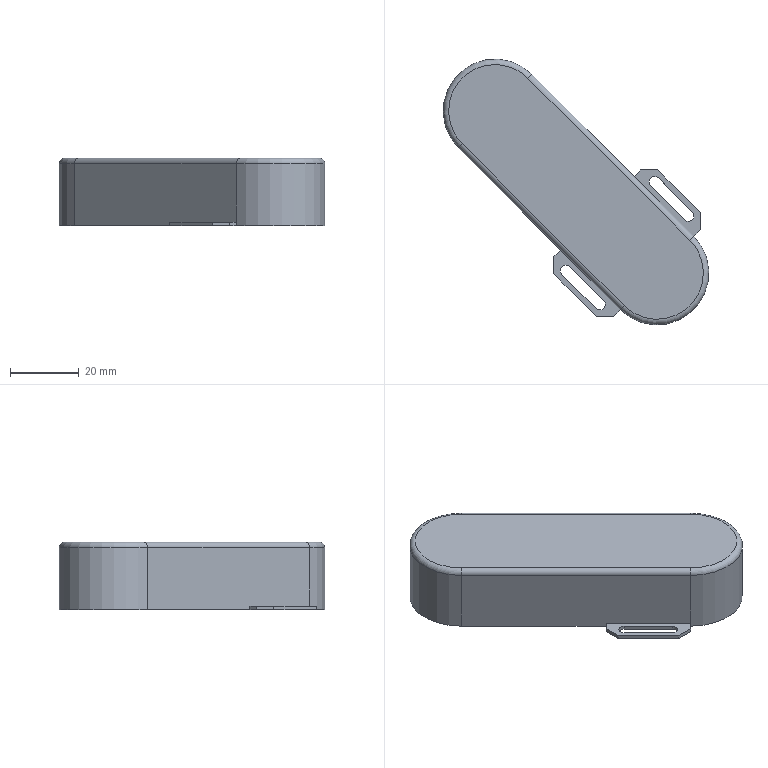Part | SolidWorks | features SplitBody 1 | 1 solid | 42 faces | box 77.123 x 77.123 x 19.6 mm | volume 7300 mm3 | plane 26 | cylinder 12 | torus 4 | commonest cylinder face diameters 3.15 x4 1.031 x2 3.131 x2 28 x2 30.1 x2
STEP:
#1=CARTESIAN_POINT('',(-32.023,223.663,-251.716));
#2=VERTEX_POINT('',#1);
#3=CARTESIAN_POINT('',(-32.023,223.663,-250.666));
#4=VERTEX_POINT('',#3);
#5=CARTESIAN_POINT('',(-32.023,223.663,-251.716));
#6=DIRECTION('',(0.,0.,1.));
#7=VECTOR('',#6,1000.);
#8=LINE('',#5,#7);
#9=EDGE_CURVE('',#2,#4,#8,.T.);
#10=ORIENTED_EDGE('',*,*,#9,.F.);
#11=CARTESIAN_POINT('',(-61.721,253.362,-251.716));
#12=VERTEX_POINT('',#11);
#13=CARTESIAN_POINT('',(-61.721,253.362,-251.716));
#14=DIRECTION('',(0.7071,-0.7071,0.));
#15=VECTOR('',#14,1000.);
#16=LINE('',#13,#15);
#17=EDGE_CURVE('',#12,#2,#16,.T.);
#18=ORIENTED_EDGE('',*,*,#17,.F.);
#19=CARTESIAN_POINT('',(-61.721,253.362,-233.681));
#20=VERTEX_POINT('',#19);
#21=CARTESIAN_POINT('',(-61.721,253.362,-233.166));
#22=DIRECTION('',(0.,0.,-1.));
#23=VECTOR('',#22,1000.);
#24=LINE('',#21,#23);
#25=EDGE_CURVE('',#20,#12,#24,.T.);
#26=ORIENTED_EDGE('',*,*,#25,.F.);
#27=CARTESIAN_POINT('',(-14.699,206.339,-233.681));
#28=VERTEX_POINT('',#27);
#29=CARTESIAN_POINT('',(-61.721,253.362,-233.681));
#30=DIRECTION('',(0.7071,-0.7071,0.));
#31=VECTOR('',#30,1000.);
#32=LINE('',#29,#31);
#33=EDGE_CURVE('',#20,#28,#32,.T.);
#34=ORIENTED_EDGE('',*,*,#33,.T.);
#35=CARTESIAN_POINT('',(-14.699,206.339,-250.666));
#36=VERTEX_POINT('',#35);
#37=CARTESIAN_POINT('',(-14.699,206.339,-233.166));
#38=DIRECTION('',(0.,0.,-1.));
#39=VECTOR('',#38,1000.);
#40=LINE('',#37,#39);
#41=EDGE_CURVE('',#28,#36,#40,.T.);
#42=ORIENTED_EDGE('',*,*,#41,.T.);
#43=CARTESIAN_POINT('',(-32.023,223.663,-250.666));
#44=DIRECTION('',(0.7071,-0.7071,0.));
#45=VECTOR('',#44,1000.);
#46=LINE('',#43,#45);
#47=EDGE_CURVE('',#4,#36,#46,.T.);
#48=ORIENTED_EDGE('',*,*,#47,.F.);
#49=EDGE_LOOP('',(#10,#18,#26,#34,#42,#48));
#50=FACE_OUTER_BOUND('',#49,.T.);
#51=CARTESIAN_POINT('',(-61.721,253.362,-233.166));
#52=DIRECTION('',(-0.7071,-0.7071,0.));
#53=DIRECTION('',(0.,0.,1.));
#54=AXIS2_PLACEMENT_3D('',#51,#52,#53);
#55=PLANE('',#54);
#56=ADVANCED_FACE('',(#50),#55,.F.);
#57=CARTESIAN_POINT('',(-35.983,185.055,-250.666));
#58=VERTEX_POINT('',#57);
#59=CARTESIAN_POINT('',(-53.307,202.379,-250.666));
#60=VERTEX_POINT('',#59);
#61=CARTESIAN_POINT('',(-53.307,202.379,-250.666));
#62=DIRECTION('',(-0.7071,0.7071,0.));
#63=VECTOR('',#62,1000.);
#64=LINE('',#61,#63);
#65=EDGE_CURVE('',#58,#60,#64,.T.);
#66=ORIENTED_EDGE('',*,*,#65,.F.);
#67=CARTESIAN_POINT('',(-35.983,185.055,-233.681));
#68=VERTEX_POINT('',#67);
#69=CARTESIAN_POINT('',(-35.983,185.055,-233.166));
#70=DIRECTION('',(0.,0.,-1.));
#71=VECTOR('',#70,1000.);
#72=LINE('',#69,#71);
#73=EDGE_CURVE('',#68,#58,#72,.T.);
#74=ORIENTED_EDGE('',*,*,#73,.F.);
#75=CARTESIAN_POINT('',(-83.005,232.078,-233.681));
#76=VERTEX_POINT('',#75);
#77=CARTESIAN_POINT('',(-35.983,185.055,-233.681));
#78=DIRECTION('',(-0.7071,0.7071,0.));
#79=VECTOR('',#78,1000.);
#80=LINE('',#77,#79);
#81=EDGE_CURVE('',#68,#76,#80,.T.);
#82=ORIENTED_EDGE('',*,*,#81,.T.);
#83=CARTESIAN_POINT('',(-83.005,232.078,-251.716));
#84=VERTEX_POINT('',#83);
#85=CARTESIAN_POINT('',(-83.005,232.078,-233.166));
#86=DIRECTION('',(0.,0.,-1.));
#87=VECTOR('',#86,1000.);
#88=LINE('',#85,#87);
#89=EDGE_CURVE('',#76,#84,#88,.T.);
#90=ORIENTED_EDGE('',*,*,#89,.T.);
#91=CARTESIAN_POINT('',(-53.307,202.379,-251.716));
#92=VERTEX_POINT('',#91);
#93=CARTESIAN_POINT('',(-35.983,185.055,-251.716));
#94=DIRECTION('',(-0.7071,0.7071,0.));
#95=VECTOR('',#94,1000.);
#96=LINE('',#93,#95);
#97=EDGE_CURVE('',#92,#84,#96,.T.);
#98=ORIENTED_EDGE('',*,*,#97,.F.);
#99=CARTESIAN_POINT('',(-53.307,202.379,-251.716));
#100=DIRECTION('',(0.,0.,-1.));
#101=VECTOR('',#100,1000.);
#102=LINE('',#99,#101);
#103=EDGE_CURVE('',#60,#92,#102,.T.);
#104=ORIENTED_EDGE('',*,*,#103,.F.);
#105=EDGE_LOOP('',(#66,#74,#82,#90,#98,#104));
#106=FACE_OUTER_BOUND('',#105,.T.);
#107=CARTESIAN_POINT('',(-35.983,185.055,-233.166));
#108=DIRECTION('',(0.7071,0.7071,0.));
#109=DIRECTION('',(0.,0.,-1.));
#110=AXIS2_PLACEMENT_3D('',#107,#108,#109);
#111=PLANE('',#110);
#112=ADVANCED_FACE('',(#106),#111,.F.);
#113=CARTESIAN_POINT('',(-82.263,232.82,-251.716));
#114=VERTEX_POINT('',#113);
#115=CARTESIAN_POINT('',(-82.263,232.82,-251.716));
#116=DIRECTION('',(0.7071,0.7071,0.));
#117=VECTOR('',#116,1000.);
#118=LINE('',#115,#117);
#119=EDGE_CURVE('',#84,#114,#118,.T.);
#120=ORIENTED_EDGE('',*,*,#119,.F.);
#121=CARTESIAN_POINT('',(-72.363,242.72,-251.716));
#122=DIRECTION('',(0.,0.,-1.));
#123=DIRECTION('',(-0.7071,-0.7071,0.));
#124=AXIS2_PLACEMENT_3D('',#121,#122,#123);
#125=CIRCLE('',#124,15.05);
#126=EDGE_CURVE('',#84,#12,#125,.T.);
#127=ORIENTED_EDGE('',*,*,#126,.T.);
#128=CARTESIAN_POINT('',(-62.464,252.619,-251.716));
#129=VERTEX_POINT('',#128);
#130=CARTESIAN_POINT('',(-62.464,252.619,-251.716));
#131=DIRECTION('',(-0.7071,-0.7071,0.));
#132=VECTOR('',#131,1000.);
#133=LINE('',#130,#132);
#134=EDGE_CURVE('',#12,#129,#133,.T.);
#135=ORIENTED_EDGE('',*,*,#134,.T.);
#136=CARTESIAN_POINT('',(-72.363,242.72,-251.716));
#137=DIRECTION('',(0.,0.,-1.));
#138=DIRECTION('',(-0.7071,-0.7071,0.));
#139=AXIS2_PLACEMENT_3D('',#136,#137,#138);
#140=CIRCLE('',#139,14.);
#141=EDGE_CURVE('',#114,#129,#140,.T.);
#142=ORIENTED_EDGE('',*,*,#141,.F.);
#143=EDGE_LOOP('',(#120,#127,#135,#142));
#144=FACE_OUTER_BOUND('',#143,.T.);
#145=CARTESIAN_POINT('',(-72.363,242.72,-251.716));
#146=DIRECTION('',(0.,0.,1.));
#147=DIRECTION('',(0.7071,0.7071,0.));
#148=AXIS2_PLACEMENT_3D('',#145,#146,#147);
#149=PLANE('',#148);
#150=ADVANCED_FACE('',(#144),#149,.F.);
#151=CARTESIAN_POINT('',(-27.197,221.064,-251.716));
#152=VERTEX_POINT('',#151);
#153=CARTESIAN_POINT('',(-24.97,223.292,-251.716));
#154=VERTEX_POINT('',#153);
#155=CARTESIAN_POINT('',(-26.083,222.178,-251.716));
#156=DIRECTION('',(0.,0.,-1.));
#157=DIRECTION('',(-0.7071,-0.7071,0.));
#158=AXIS2_PLACEMENT_3D('',#155,#156,#157);
#159=CIRCLE('',#158,1.575);
#160=EDGE_CURVE('',#152,#154,#159,.T.);
#161=ORIENTED_EDGE('',*,*,#160,.F.);
#162=CARTESIAN_POINT('',(-17.297,211.165,-251.716));
#163=VERTEX_POINT('',#162);
#164=CARTESIAN_POINT('',(-60.608,254.475,-251.716));
#165=DIRECTION('',(-0.7071,0.7071,0.));
#166=VECTOR('',#165,1000.);
#167=LINE('',#164,#166);
#168=EDGE_CURVE('',#163,#152,#167,.T.);
#169=ORIENTED_EDGE('',*,*,#168,.F.);
#170=CARTESIAN_POINT('',(-15.07,213.392,-251.716));
#171=VERTEX_POINT('',#170);
#172=CARTESIAN_POINT('',(-16.184,212.279,-251.716));
#173=DIRECTION('',(0.,0.,-1.));
#174=DIRECTION('',(-0.7071,-0.7071,0.));
#175=AXIS2_PLACEMENT_3D('',#172,#173,#174);
#176=CIRCLE('',#175,1.575);
#177=EDGE_CURVE('',#171,#163,#176,.T.);
#178=ORIENTED_EDGE('',*,*,#177,.F.);
#179=CARTESIAN_POINT('',(-58.38,256.703,-251.716));
#180=DIRECTION('',(0.7071,-0.7071,0.));
#181=VECTOR('',#180,1000.);
#182=LINE('',#179,#181);
#183=EDGE_CURVE('',#154,#171,#182,.T.);
#184=ORIENTED_EDGE('',*,*,#183,.F.);
#185=EDGE_LOOP('',(#161,#169,#178,#184));
#186=FACE_BOUND('',#185,.T.);
#187=CARTESIAN_POINT('',(-30.043,225.643,-251.716));
#188=VERTEX_POINT('',#187);
#189=CARTESIAN_POINT('',(-27.568,228.118,-251.716));
#190=DIRECTION('',(-0.7071,-0.7071,0.));
#191=VECTOR('',#190,1000.);
#192=LINE('',#189,#191);
#193=EDGE_CURVE('',#188,#2,#192,.T.);
#194=ORIENTED_EDGE('',*,*,#193,.F.);
#195=CARTESIAN_POINT('',(-25.093,225.643,-251.716));
#196=VERTEX_POINT('',#195);
#197=CARTESIAN_POINT('',(-62.464,225.643,-251.716));
#198=DIRECTION('',(1.,0.,0.));
#199=VECTOR('',#198,1000.);
#200=LINE('',#197,#199);
#201=EDGE_CURVE('',#188,#196,#200,.T.);
#202=ORIENTED_EDGE('',*,*,#201,.T.);
#203=CARTESIAN_POINT('',(-12.719,213.269,-251.716));
#204=VERTEX_POINT('',#203);
#205=CARTESIAN_POINT('',(-10.244,210.794,-251.716));
#206=DIRECTION('',(-0.7071,0.7071,0.));
#207=VECTOR('',#206,1000.);
#208=LINE('',#205,#207);
#209=EDGE_CURVE('',#204,#196,#208,.T.);
#210=ORIENTED_EDGE('',*,*,#209,.F.);
#211=CARTESIAN_POINT('',(-12.719,208.319,-251.716));
#212=VERTEX_POINT('',#211);
#213=CARTESIAN_POINT('',(-12.719,252.619,-251.716));
#214=DIRECTION('',(0.,-1.,0.));
#215=VECTOR('',#214,1000.);
#216=LINE('',#213,#215);
#217=EDGE_CURVE('',#204,#212,#216,.T.);
#218=ORIENTED_EDGE('',*,*,#217,.T.);
#219=CARTESIAN_POINT('',(-14.699,206.339,-251.716));
#220=VERTEX_POINT('',#219);
#221=CARTESIAN_POINT('',(-10.244,210.794,-251.716));
#222=DIRECTION('',(-0.7071,-0.7071,0.));
#223=VECTOR('',#222,1000.);
#224=LINE('',#221,#223);
#225=EDGE_CURVE('',#212,#220,#224,.T.);
#226=ORIENTED_EDGE('',*,*,#225,.T.);
#227=CARTESIAN_POINT('',(-15.441,205.597,-251.716));
#228=VERTEX_POINT('',#227);
#229=CARTESIAN_POINT('',(-15.441,205.597,-251.716));
#230=DIRECTION('',(-0.7071,-0.7071,0.));
#231=VECTOR('',#230,1000.);
#232=LINE('',#229,#231);
#233=EDGE_CURVE('',#220,#228,#232,.T.);
#234=ORIENTED_EDGE('',*,*,#233,.T.);
#235=CARTESIAN_POINT('',(-62.464,252.619,-251.716));
#236=DIRECTION('',(0.7071,-0.7071,0.));
#237=VECTOR('',#236,1000.);
#238=LINE('',#235,#237);
#239=EDGE_CURVE('',#129,#228,#238,.T.);
#240=ORIENTED_EDGE('',*,*,#239,.F.);
#241=ORIENTED_EDGE('',*,*,#134,.F.);
#242=ORIENTED_EDGE('',*,*,#17,.T.);
#243=EDGE_LOOP('',(#194,#202,#210,#218,#226,#234,#240,#241,#242));
#244=FACE_OUTER_BOUND('',#243,.T.);
#245=CARTESIAN_POINT('',(-62.464,252.619,-251.716));
#246=DIRECTION('',(0.,0.,-1.));
#247=DIRECTION('',(0.7071,-0.7071,0.));
#248=AXIS2_PLACEMENT_3D('',#245,#246,#247);
#249=PLANE('',#248);
#250=ADVANCED_FACE('',(#186,#244),#249,.T.);
#251=ORIENTED_EDGE('',*,*,#233,.F.);
#252=CARTESIAN_POINT('',(-35.983,185.055,-251.716));
#253=VERTEX_POINT('',#252);
#254=CARTESIAN_POINT('',(-25.341,195.697,-251.716));
#255=DIRECTION('',(0.,0.,-1.));
#256=DIRECTION('',(-0.7071,-0.7071,0.));
#257=AXIS2_PLACEMENT_3D('',#254,#255,#256);
#258=CIRCLE('',#257,15.05);
#259=EDGE_CURVE('',#220,#253,#258,.T.);
#260=ORIENTED_EDGE('',*,*,#259,.T.);
#261=CARTESIAN_POINT('',(-35.24,185.798,-251.716));
#262=VERTEX_POINT('',#261);
#263=CARTESIAN_POINT('',(-35.24,185.798,-251.716));
#264=DIRECTION('',(0.7071,0.7071,0.));
#265=VECTOR('',#264,1000.);
#266=LINE('',#263,#265);
#267=EDGE_CURVE('',#253,#262,#266,.T.);
#268=ORIENTED_EDGE('',*,*,#267,.T.);
#269=CARTESIAN_POINT('',(-25.341,195.697,-251.716));
#270=DIRECTION('',(0.,0.,-1.));
#271=DIRECTION('',(0.7071,0.7071,0.));
#272=AXIS2_PLACEMENT_3D('',#269,#270,#271);
#273=CIRCLE('',#272,14.);
#274=EDGE_CURVE('',#228,#262,#273,.T.);
#275=ORIENTED_EDGE('',*,*,#274,.F.);
#276=EDGE_LOOP('',(#251,#260,#268,#275));
#277=FACE_OUTER_BOUND('',#276,.T.);
#278=CARTESIAN_POINT('',(-25.341,195.697,-251.716));
#279=DIRECTION('',(0.,0.,1.));
#280=DIRECTION('',(0.7071,0.7071,0.));
#281=AXIS2_PLACEMENT_3D('',#278,#279,#280);
#282=PLANE('',#281);
#283=ADVANCED_FACE('',(#277),#282,.F.);
#284=CARTESIAN_POINT('',(-35.24,185.798,-233.681));
#285=VERTEX_POINT('',#284);
#286=CARTESIAN_POINT('',(-82.263,232.82,-233.681));
#287=VERTEX_POINT('',#286);
#288=CARTESIAN_POINT('',(-35.24,185.798,-233.681));
#289=DIRECTION('',(-0.7071,0.7071,0.));
#290=VECTOR('',#289,1000.);
#291=LINE('',#288,#290);
#292=EDGE_CURVE('',#285,#287,#291,.T.);
#293=ORIENTED_EDGE('',*,*,#292,.T.);
#294=CARTESIAN_POINT('',(-81.898,233.185,-233.166));
#295=VERTEX_POINT('',#294);
#296=CARTESIAN_POINT('',(-81.898,233.185,-233.681));
#297=DIRECTION('',(0.7071,-0.7071,0.));
#298=DIRECTION('',(0.,0.,-1.));
#299=AXIS2_PLACEMENT_3D('',#296,#297,#298);
#300=CIRCLE('',#299,0.5156);
#301=EDGE_CURVE('',#295,#287,#300,.T.);
#302=ORIENTED_EDGE('',*,*,#301,.F.);
#303=CARTESIAN_POINT('',(-34.876,186.162,-233.166));
#304=VERTEX_POINT('',#303);
#305=CARTESIAN_POINT('',(-34.876,186.162,-233.166));
#306=DIRECTION('',(-0.7071,0.7071,0.));
#307=VECTOR('',#306,1000.);
#308=LINE('',#305,#307);
#309=EDGE_CURVE('',#304,#295,#308,.T.);
#310=ORIENTED_EDGE('',*,*,#309,.F.);
#311=CARTESIAN_POINT('',(-34.876,186.162,-233.681));
#312=DIRECTION('',(0.7071,-0.7071,0.));
#313=DIRECTION('',(0.,0.,-1.));
#314=AXIS2_PLACEMENT_3D('',#311,#312,#313);
#315=CIRCLE('',#314,0.5156);
#316=EDGE_CURVE('',#304,#285,#315,.T.);
#317=ORIENTED_EDGE('',*,*,#316,.T.);
#318=EDGE_LOOP('',(#293,#302,#310,#317));
#319=FACE_OUTER_BOUND('',#318,.T.);
#320=CARTESIAN_POINT('',(-34.876,186.162,-233.681));
#321=DIRECTION('',(-0.7071,0.7071,0.));
#322=DIRECTION('',(0.,0.,-1.));
#323=AXIS2_PLACEMENT_3D('',#320,#321,#322);
#324=CYLINDRICAL_SURFACE('',#323,0.5156);
#325=ADVANCED_FACE('',(#319),#324,.F.);
#326=CARTESIAN_POINT('',(-35.24,185.798,-251.716));
#327=DIRECTION('',(-0.7071,0.7071,0.));
#328=VECTOR('',#327,1000.);
#329=LINE('',#326,#328);
#330=EDGE_CURVE('',#262,#114,#329,.T.);
#331=ORIENTED_EDGE('',*,*,#330,.T.);
#332=CARTESIAN_POINT('',(-82.263,232.82,-233.166));
#333=DIRECTION('',(0.,0.,-1.));
#334=VECTOR('',#333,1000.);
#335=LINE('',#332,#334);
#336=EDGE_CURVE('',#287,#114,#335,.T.);
#337=ORIENTED_EDGE('',*,*,#336,.F.);
#338=ORIENTED_EDGE('',*,*,#292,.F.);
#339=CARTESIAN_POINT('',(-35.24,185.798,-233.166));
#340=DIRECTION('',(0.,0.,-1.));
#341=VECTOR('',#340,1000.);
#342=LINE('',#339,#341);
#343=EDGE_CURVE('',#285,#262,#342,.T.);
#344=ORIENTED_EDGE('',*,*,#343,.T.);
#345=EDGE_LOOP('',(#331,#337,#338,#344));
#346=FACE_OUTER_BOUND('',#345,.T.);
#347=CARTESIAN_POINT('',(-35.24,185.798,-233.166));
#348=DIRECTION('',(0.7071,0.7071,0.));
#349=DIRECTION('',(0.,0.,-1.));
#350=AXIS2_PLACEMENT_3D('',#347,#348,#349);
#351=PLANE('',#350);
#352=ADVANCED_FACE('',(#346),#351,.T.);
#353=CARTESIAN_POINT('',(-62.464,252.619,-233.681));
#354=VERTEX_POINT('',#353);
#355=CARTESIAN_POINT('',(-72.363,242.72,-233.681));
#356=DIRECTION('',(0.,0.,-1.));
#357=DIRECTION('',(-0.7071,-0.7071,0.));
#358=AXIS2_PLACEMENT_3D('',#355,#356,#357);
#359=CIRCLE('',#358,14.);
#360=EDGE_CURVE('',#287,#354,#359,.T.);
#361=ORIENTED_EDGE('',*,*,#360,.T.);
#362=CARTESIAN_POINT('',(-62.829,252.255,-233.166));
#363=VERTEX_POINT('',#362);
#364=CARTESIAN_POINT('',(-62.829,252.255,-233.681));
#365=DIRECTION('',(-0.7071,0.7071,0.));
#366=DIRECTION('',(0.,0.,-1.));
#367=AXIS2_PLACEMENT_3D('',#364,#365,#366);
#368=CIRCLE('',#367,0.5156);
#369=EDGE_CURVE('',#363,#354,#368,.T.);
#370=ORIENTED_EDGE('',*,*,#369,.F.);
#371=CARTESIAN_POINT('',(-72.363,242.72,-233.166));
#372=DIRECTION('',(0.,0.,-1.));
#373=DIRECTION('',(-0.7071,-0.7071,0.));
#374=AXIS2_PLACEMENT_3D('',#371,#372,#373);
#375=CIRCLE('',#374,13.484);
#376=EDGE_CURVE('',#295,#363,#375,.T.);
#377=ORIENTED_EDGE('',*,*,#376,.F.);
#378=ORIENTED_EDGE('',*,*,#301,.T.);
#379=EDGE_LOOP('',(#361,#370,#377,#378));
#380=FACE_OUTER_BOUND('',#379,.T.);
#381=CARTESIAN_POINT('',(-72.363,242.72,-233.681));
#382=DIRECTION('',(0.,0.,-1.));
#383=DIRECTION('',(-0.7071,-0.7071,0.));
#384=AXIS2_PLACEMENT_3D('',#381,#382,#383);
#385=TOROIDAL_SURFACE('',#384,13.484,0.5156);
#386=ADVANCED_FACE('',(#380),#385,.F.);
#387=ORIENTED_EDGE('',*,*,#141,.T.);
#388=CARTESIAN_POINT('',(-62.464,252.619,-233.166));
#389=DIRECTION('',(0.,0.,-1.));
#390=VECTOR('',#389,1000.);
#391=LINE('',#388,#390);
#392=EDGE_CURVE('',#354,#129,#391,.T.);
#393=ORIENTED_EDGE('',*,*,#392,.F.);
#394=ORIENTED_EDGE('',*,*,#360,.F.);
#395=ORIENTED_EDGE('',*,*,#336,.T.);
#396=EDGE_LOOP('',(#387,#393,#394,#395));
#397=FACE_OUTER_BOUND('',#396,.T.);
#398=CARTESIAN_POINT('',(-72.363,242.72,-233.166));
#399=DIRECTION('',(0.,0.,-1.));
#400=DIRECTION('',(-0.7071,-0.7071,0.));
#401=AXIS2_PLACEMENT_3D('',#398,#399,#400);
#402=CYLINDRICAL_SURFACE('',#401,14.);
#403=ADVANCED_FACE('',(#397),#402,.F.);
#404=CARTESIAN_POINT('',(-15.441,205.597,-233.681));
#405=VERTEX_POINT('',#404);
#406=CARTESIAN_POINT('',(-62.464,252.619,-233.681));
#407=DIRECTION('',(0.7071,-0.7071,0.));
#408=VECTOR('',#407,1000.);
#409=LINE('',#406,#408);
#410=EDGE_CURVE('',#354,#405,#409,.T.);
#411=ORIENTED_EDGE('',*,*,#410,.T.);
#412=CARTESIAN_POINT('',(-15.806,205.232,-233.166));
#413=VERTEX_POINT('',#412);
#414=CARTESIAN_POINT('',(-15.806,205.232,-233.681));
#415=DIRECTION('',(-0.7071,0.7071,0.));
#416=DIRECTION('',(0.,0.,-1.));
#417=AXIS2_PLACEMENT_3D('',#414,#415,#416);
#418=CIRCLE('',#417,0.5156);
#419=EDGE_CURVE('',#413,#405,#418,.T.);
#420=ORIENTED_EDGE('',*,*,#419,.F.);
#421=CARTESIAN_POINT('',(-62.829,252.255,-233.166));
#422=DIRECTION('',(0.7071,-0.7071,0.));
#423=VECTOR('',#422,1000.);
#424=LINE('',#421,#423);
#425=EDGE_CURVE('',#363,#413,#424,.T.);
#426=ORIENTED_EDGE('',*,*,#425,.F.);
#427=ORIENTED_EDGE('',*,*,#369,.T.);
#428=EDGE_LOOP('',(#411,#420,#426,#427));
#429=FACE_OUTER_BOUND('',#428,.T.);
#430=CARTESIAN_POINT('',(-62.829,252.255,-233.681));
#431=DIRECTION('',(0.7071,-0.7071,0.));
#432=DIRECTION('',(0.,0.,1.));
#433=AXIS2_PLACEMENT_3D('',#430,#431,#432);
#434=CYLINDRICAL_SURFACE('',#433,0.5156);
#435=ADVANCED_FACE('',(#429),#434,.F.);
#436=ORIENTED_EDGE('',*,*,#239,.T.);
#437=CARTESIAN_POINT('',(-15.441,205.597,-233.166));
#438=DIRECTION('',(0.,0.,-1.));
#439=VECTOR('',#438,1000.);
#440=LINE('',#437,#439);
#441=EDGE_CURVE('',#405,#228,#440,.T.);
#442=ORIENTED_EDGE('',*,*,#441,.F.);
#443=ORIENTED_EDGE('',*,*,#410,.F.);
#444=ORIENTED_EDGE('',*,*,#392,.T.);
#445=EDGE_LOOP('',(#436,#442,#443,#444));
#446=FACE_OUTER_BOUND('',#445,.T.);
#447=CARTESIAN_POINT('',(-62.464,252.619,-233.166));
#448=DIRECTION('',(-0.7071,-0.7071,0.));
#449=DIRECTION('',(0.,0.,1.));
#450=AXIS2_PLACEMENT_3D('',#447,#448,#449);
#451=PLANE('',#450);
#452=ADVANCED_FACE('',(#446),#451,.T.);
#453=CARTESIAN_POINT('',(-25.341,195.697,-233.166));
#454=DIRECTION('',(0.,0.,-1.));
#455=DIRECTION('',(0.7071,0.7071,0.));
#456=AXIS2_PLACEMENT_3D('',#453,#454,#455);
#457=CIRCLE('',#456,13.484);
#458=EDGE_CURVE('',#413,#304,#457,.T.);
#459=ORIENTED_EDGE('',*,*,#458,.F.);
#460=ORIENTED_EDGE('',*,*,#419,.T.);
#461=CARTESIAN_POINT('',(-25.341,195.697,-233.681));
#462=DIRECTION('',(0.,0.,-1.));
#463=DIRECTION('',(0.7071,0.7071,0.));
#464=AXIS2_PLACEMENT_3D('',#461,#462,#463);
#465=CIRCLE('',#464,14.);
#466=EDGE_CURVE('',#405,#285,#465,.T.);
#467=ORIENTED_EDGE('',*,*,#466,.T.);
#468=ORIENTED_EDGE('',*,*,#316,.F.);
#469=EDGE_LOOP('',(#459,#460,#467,#468));
#470=FACE_OUTER_BOUND('',#469,.T.);
#471=CARTESIAN_POINT('',(-25.341,195.697,-233.681));
#472=DIRECTION('',(0.,0.,-1.));
#473=DIRECTION('',(-0.7071,-0.7071,0.));
#474=AXIS2_PLACEMENT_3D('',#471,#472,#473);
#475=TOROIDAL_SURFACE('',#474,13.484,0.5156);
#476=ADVANCED_FACE('',(#470),#475,.F.);
#477=ORIENTED_EDGE('',*,*,#466,.F.);
#478=ORIENTED_EDGE('',*,*,#441,.T.);
#479=ORIENTED_EDGE('',*,*,#274,.T.);
#480=ORIENTED_EDGE('',*,*,#343,.F.);
#481=EDGE_LOOP('',(#477,#478,#479,#480));
#482=FACE_OUTER_BOUND('',#481,.T.);
#483=CARTESIAN_POINT('',(-25.341,195.697,-233.166));
#484=DIRECTION('',(0.,0.,-1.));
#485=DIRECTION('',(-0.7071,-0.7071,0.));
#486=AXIS2_PLACEMENT_3D('',#483,#484,#485);
#487=CYLINDRICAL_SURFACE('',#486,14.);
#488=ADVANCED_FACE('',(#482),#487,.F.);
#489=CARTESIAN_POINT('',(-52.936,195.326,-251.716));
#490=VERTEX_POINT('',#489);
#491=CARTESIAN_POINT('',(-50.708,197.553,-251.716));
#492=VERTEX_POINT('',#491);
#493=CARTESIAN_POINT('',(-51.822,196.439,-251.716));
#494=DIRECTION('',(0.,0.,-1.));
#495=DIRECTION('',(-0.7071,-0.7071,0.));
#496=AXIS2_PLACEMENT_3D('',#493,#494,#495);
#497=CIRCLE('',#496,1.575);
#498=EDGE_CURVE('',#490,#492,#497,.T.);
#499=ORIENTED_EDGE('',*,*,#498,.F.);
#500=CARTESIAN_POINT('',(-43.036,185.426,-251.716));
#501=VERTEX_POINT('',#500);
#502=CARTESIAN_POINT('',(-39.324,181.714,-251.716));
#503=DIRECTION('',(-0.7071,0.7071,0.));
#504=VECTOR('',#503,1000.);
#505=LINE('',#502,#504);
#506=EDGE_CURVE('',#501,#490,#505,.T.);
#507=ORIENTED_EDGE('',*,*,#506,.F.);
#508=CARTESIAN_POINT('',(-40.809,187.654,-251.716));
#509=VERTEX_POINT('',#508);
#510=CARTESIAN_POINT('',(-41.922,186.54,-251.716));
#511=DIRECTION('',(0.,0.,-1.));
#512=DIRECTION('',(-0.7071,-0.7071,0.));
#513=AXIS2_PLACEMENT_3D('',#510,#511,#512);
#514=CIRCLE('',#513,1.575);
#515=EDGE_CURVE('',#509,#501,#514,.T.);
#516=ORIENTED_EDGE('',*,*,#515,.F.);
#517=CARTESIAN_POINT('',(-37.096,183.941,-251.716));
#518=DIRECTION('',(0.7071,-0.7071,0.));
#519=VECTOR('',#518,1000.);
#520=LINE('',#517,#519);
#521=EDGE_CURVE('',#492,#509,#520,.T.);
#522=ORIENTED_EDGE('',*,*,#521,.F.);
#523=EDGE_LOOP('',(#499,#507,#516,#522));
#524=FACE_BOUND('',#523,.T.);
#525=CARTESIAN_POINT('',(-55.287,195.45,-251.716));
#526=VERTEX_POINT('',#525);
#527=CARTESIAN_POINT('',(-42.912,183.075,-251.716));
#528=VERTEX_POINT('',#527);
#529=CARTESIAN_POINT('',(-57.762,197.924,-251.716));
#530=DIRECTION('',(0.7071,-0.7071,0.));
#531=VECTOR('',#530,1000.);
#532=LINE('',#529,#531);
#533=EDGE_CURVE('',#526,#528,#532,.T.);
#534=ORIENTED_EDGE('',*,*,#533,.F.);
#535=CARTESIAN_POINT('',(-55.287,200.399,-251.716));
#536=VERTEX_POINT('',#535);
#537=CARTESIAN_POINT('',(-55.287,185.798,-251.716));
#538=DIRECTION('',(0.,1.,0.));
#539=VECTOR('',#538,1000.);
#540=LINE('',#537,#539);
#541=EDGE_CURVE('',#526,#536,#540,.T.);
#542=ORIENTED_EDGE('',*,*,#541,.T.);
#543=CARTESIAN_POINT('',(-57.762,197.924,-251.716));
#544=DIRECTION('',(0.7071,0.7071,0.));
#545=VECTOR('',#544,1000.);
#546=LINE('',#543,#545);
#547=EDGE_CURVE('',#536,#92,#546,.T.);
#548=ORIENTED_EDGE('',*,*,#547,.T.);
#549=ORIENTED_EDGE('',*,*,#97,.T.);
#550=ORIENTED_EDGE('',*,*,#119,.T.);
#551=ORIENTED_EDGE('',*,*,#330,.F.);
#552=ORIENTED_EDGE('',*,*,#267,.F.);
#553=CARTESIAN_POINT('',(-37.963,183.075,-251.716));
#554=VERTEX_POINT('',#553);
#555=CARTESIAN_POINT('',(-40.438,180.6,-251.716));
#556=DIRECTION('',(0.7071,0.7071,0.));
#557=VECTOR('',#556,1000.);
#558=LINE('',#555,#557);
#559=EDGE_CURVE('',#554,#253,#558,.T.);
#560=ORIENTED_EDGE('',*,*,#559,.F.);
#561=CARTESIAN_POINT('',(-35.24,183.075,-251.716));
#562=DIRECTION('',(-1.,0.,0.));
#563=VECTOR('',#562,1000.);
#564=LINE('',#561,#563);
#565=EDGE_CURVE('',#554,#528,#564,.T.);
#566=ORIENTED_EDGE('',*,*,#565,.T.);
#567=EDGE_LOOP('',(#534,#542,#548,#549,#550,#551,#552,#560,#566));
#568=FACE_OUTER_BOUND('',#567,.T.);
#569=CARTESIAN_POINT('',(-35.24,185.798,-251.716));
#570=DIRECTION('',(0.,0.,-1.));
#571=DIRECTION('',(-0.7071,0.7071,0.));
#572=AXIS2_PLACEMENT_3D('',#569,#570,#571);
#573=PLANE('',#572);
#574=ADVANCED_FACE('',(#524,#568),#573,.T.);
#575=CARTESIAN_POINT('',(-25.341,195.697,-233.681));
#576=DIRECTION('',(0.,0.,-1.));
#577=DIRECTION('',(-0.7071,-0.7071,0.));
#578=AXIS2_PLACEMENT_3D('',#575,#576,#577);
#579=CIRCLE('',#578,15.05);
#580=EDGE_CURVE('',#28,#68,#579,.T.);
#581=ORIENTED_EDGE('',*,*,#580,.T.);
#582=ORIENTED_EDGE('',*,*,#73,.T.);
#583=CARTESIAN_POINT('',(-35.983,185.055,-251.716));
#584=DIRECTION('',(0.,0.,1.));
#585=VECTOR('',#584,1000.);
#586=LINE('',#583,#585);
#587=EDGE_CURVE('',#253,#58,#586,.T.);
#588=ORIENTED_EDGE('',*,*,#587,.F.);
#589=ORIENTED_EDGE('',*,*,#259,.F.);
#590=CARTESIAN_POINT('',(-14.699,206.339,-250.666));
#591=DIRECTION('',(0.,0.,-1.));
#592=VECTOR('',#591,1000.);
#593=LINE('',#590,#592);
#594=EDGE_CURVE('',#36,#220,#593,.T.);
#595=ORIENTED_EDGE('',*,*,#594,.F.);
#596=ORIENTED_EDGE('',*,*,#41,.F.);
#597=EDGE_LOOP('',(#581,#582,#588,#589,#595,#596));
#598=FACE_OUTER_BOUND('',#597,.T.);
#599=CARTESIAN_POINT('',(-25.341,195.697,-233.166));
#600=DIRECTION('',(0.,0.,-1.));
#601=DIRECTION('',(-0.7071,-0.7071,0.));
#602=AXIS2_PLACEMENT_3D('',#599,#600,#601);
#603=CYLINDRICAL_SURFACE('',#602,15.05);
#604=ADVANCED_FACE('',(#598),#603,.T.);
#605=CARTESIAN_POINT('',(-15.806,205.232,-232.116));
#606=VERTEX_POINT('',#605);
#607=CARTESIAN_POINT('',(-34.876,186.162,-232.116));
#608=VERTEX_POINT('',#607);
#609=CARTESIAN_POINT('',(-25.341,195.697,-232.116));
#610=DIRECTION('',(0.,0.,-1.));
#611=DIRECTION('',(-0.7071,-0.7071,0.));
#612=AXIS2_PLACEMENT_3D('',#609,#610,#611);
#613=CIRCLE('',#612,13.484);
#614=EDGE_CURVE('',#606,#608,#613,.T.);
#615=ORIENTED_EDGE('',*,*,#614,.T.);
#616=CARTESIAN_POINT('',(-34.876,186.162,-233.681));
#617=DIRECTION('',(0.7071,-0.7071,0.));
#618=DIRECTION('',(0.,0.,-1.));
#619=AXIS2_PLACEMENT_3D('',#616,#617,#618);
#620=CIRCLE('',#619,1.566);
#621=EDGE_CURVE('',#608,#68,#620,.T.);
#622=ORIENTED_EDGE('',*,*,#621,.T.);
#623=ORIENTED_EDGE('',*,*,#580,.F.);
#624=CARTESIAN_POINT('',(-15.806,205.232,-233.681));
#625=DIRECTION('',(-0.7071,0.7071,0.));
#626=DIRECTION('',(0.7071,0.7071,0.));
#627=AXIS2_PLACEMENT_3D('',#624,#625,#626);
#628=CIRCLE('',#627,1.566);
#629=EDGE_CURVE('',#606,#28,#628,.T.);
#630=ORIENTED_EDGE('',*,*,#629,.F.);
#631=EDGE_LOOP('',(#615,#622,#623,#630));
#632=FACE_OUTER_BOUND('',#631,.T.);
#633=CARTESIAN_POINT('',(-25.341,195.697,-233.681));
#634=DIRECTION('',(0.,0.,-1.));
#635=DIRECTION('',(-0.7071,-0.7071,0.));
#636=AXIS2_PLACEMENT_3D('',#633,#634,#635);
#637=TOROIDAL_SURFACE('',#636,13.484,1.566);
#638=ADVANCED_FACE('',(#632),#637,.T.);
#639=ORIENTED_EDGE('',*,*,#33,.F.);
#640=CARTESIAN_POINT('',(-62.829,252.255,-232.116));
#641=VERTEX_POINT('',#640);
#642=CARTESIAN_POINT('',(-62.829,252.255,-233.681));
#643=DIRECTION('',(-0.7071,0.7071,0.));
#644=DIRECTION('',(0.,0.,1.));
#645=AXIS2_PLACEMENT_3D('',#642,#643,#644);
#646=CIRCLE('',#645,1.566);
#647=EDGE_CURVE('',#641,#20,#646,.T.);
#648=ORIENTED_EDGE('',*,*,#647,.F.);
#649=CARTESIAN_POINT('',(-62.829,252.255,-232.116));
#650=DIRECTION('',(0.7071,-0.7071,0.));
#651=VECTOR('',#650,1000.);
#652=LINE('',#649,#651);
#653=EDGE_CURVE('',#641,#606,#652,.T.);
#654=ORIENTED_EDGE('',*,*,#653,.T.);
#655=ORIENTED_EDGE('',*,*,#629,.T.);
#656=EDGE_LOOP('',(#639,#648,#654,#655));
#657=FACE_OUTER_BOUND('',#656,.T.);
#658=CARTESIAN_POINT('',(-62.829,252.255,-233.681));
#659=DIRECTION('',(0.7071,-0.7071,0.));
#660=DIRECTION('',(0.,0.,1.));
#661=AXIS2_PLACEMENT_3D('',#658,#659,#660);
#662=CYLINDRICAL_SURFACE('',#661,1.566);
#663=ADVANCED_FACE('',(#657),#662,.T.);
#664=ORIENTED_EDGE('',*,*,#126,.F.);
#665=ORIENTED_EDGE('',*,*,#89,.F.);
#666=CARTESIAN_POINT('',(-72.363,242.72,-233.681));
#667=DIRECTION('',(0.,0.,-1.));
#668=DIRECTION('',(-0.7071,-0.7071,0.));
#669=AXIS2_PLACEMENT_3D('',#666,#667,#668);
#670=CIRCLE('',#669,15.05);
#671=EDGE_CURVE('',#76,#20,#670,.T.);
#672=ORIENTED_EDGE('',*,*,#671,.T.);
#673=ORIENTED_EDGE('',*,*,#25,.T.);
#674=EDGE_LOOP('',(#664,#665,#672,#673));
#675=FACE_OUTER_BOUND('',#674,.T.);
#676=CARTESIAN_POINT('',(-72.363,242.72,-233.166));
#677=DIRECTION('',(0.,0.,-1.));
#678=DIRECTION('',(-0.7071,-0.7071,0.));
#679=AXIS2_PLACEMENT_3D('',#676,#677,#678);
#680=CYLINDRICAL_SURFACE('',#679,15.05);
#681=ADVANCED_FACE('',(#675),#680,.T.);
#682=ORIENTED_EDGE('',*,*,#671,.F.);
#683=CARTESIAN_POINT('',(-81.898,233.185,-232.116));
#684=VERTEX_POINT('',#683);
#685=CARTESIAN_POINT('',(-81.898,233.185,-233.681));
#686=DIRECTION('',(0.7071,-0.7071,0.));
#687=DIRECTION('',(0.,0.,1.));
#688=AXIS2_PLACEMENT_3D('',#685,#686,#687);
#689=CIRCLE('',#688,1.566);
#690=EDGE_CURVE('',#684,#76,#689,.T.);
#691=ORIENTED_EDGE('',*,*,#690,.F.);
#692=CARTESIAN_POINT('',(-72.363,242.72,-232.116));
#693=DIRECTION('',(0.,0.,-1.));
#694=DIRECTION('',(-0.7071,-0.7071,0.));
#695=AXIS2_PLACEMENT_3D('',#692,#693,#694);
#696=CIRCLE('',#695,13.484);
#697=EDGE_CURVE('',#684,#641,#696,.T.);
#698=ORIENTED_EDGE('',*,*,#697,.T.);
#699=ORIENTED_EDGE('',*,*,#647,.T.);
#700=EDGE_LOOP('',(#682,#691,#698,#699));
#701=FACE_OUTER_BOUND('',#700,.T.);
#702=CARTESIAN_POINT('',(-72.363,242.72,-233.681));
#703=DIRECTION('',(0.,0.,-1.));
#704=DIRECTION('',(-0.7071,-0.7071,0.));
#705=AXIS2_PLACEMENT_3D('',#702,#703,#704);
#706=TOROIDAL_SURFACE('',#705,13.484,1.566);
#707=ADVANCED_FACE('',(#701),#706,.T.);
#708=ORIENTED_EDGE('',*,*,#81,.F.);
#709=ORIENTED_EDGE('',*,*,#621,.F.);
#710=CARTESIAN_POINT('',(-34.876,186.162,-232.116));
#711=DIRECTION('',(-0.7071,0.7071,0.));
#712=VECTOR('',#711,1000.);
#713=LINE('',#710,#712);
#714=EDGE_CURVE('',#608,#684,#713,.T.);
#715=ORIENTED_EDGE('',*,*,#714,.T.);
#716=ORIENTED_EDGE('',*,*,#690,.T.);
#717=EDGE_LOOP('',(#708,#709,#715,#716));
#718=FACE_OUTER_BOUND('',#717,.T.);
#719=CARTESIAN_POINT('',(-34.876,186.162,-233.681));
#720=DIRECTION('',(-0.7071,0.7071,0.));
#721=DIRECTION('',(0.,0.,-1.));
#722=AXIS2_PLACEMENT_3D('',#719,#720,#721);
#723=CYLINDRICAL_SURFACE('',#722,1.566);
#724=ADVANCED_FACE('',(#718),#723,.T.);
#725=ORIENTED_EDGE('',*,*,#425,.T.);
#726=ORIENTED_EDGE('',*,*,#458,.T.);
#727=ORIENTED_EDGE('',*,*,#309,.T.);
#728=ORIENTED_EDGE('',*,*,#376,.T.);
#729=EDGE_LOOP('',(#725,#726,#727,#728));
#730=FACE_OUTER_BOUND('',#729,.T.);
#731=CARTESIAN_POINT('',(-25.341,195.697,-233.166));
#732=DIRECTION('',(0.,0.,-1.));
#733=DIRECTION('',(-0.7071,-0.7071,0.));
#734=AXIS2_PLACEMENT_3D('',#731,#732,#733);
#735=PLANE('',#734);
#736=ADVANCED_FACE('',(#730),#735,.T.);
#737=ORIENTED_EDGE('',*,*,#614,.F.);
#738=ORIENTED_EDGE('',*,*,#653,.F.);
#739=ORIENTED_EDGE('',*,*,#697,.F.);
#740=ORIENTED_EDGE('',*,*,#714,.F.);
#741=EDGE_LOOP('',(#737,#738,#739,#740));
#742=FACE_OUTER_BOUND('',#741,.T.);
#743=CARTESIAN_POINT('',(-25.341,195.697,-232.116));
#744=DIRECTION('',(0.,0.,-1.));
#745=DIRECTION('',(-0.7071,-0.7071,0.));
#746=AXIS2_PLACEMENT_3D('',#743,#744,#745);
#747=PLANE('',#746);
#748=ADVANCED_FACE('',(#742),#747,.F.);
#749=CARTESIAN_POINT('',(-37.963,183.075,-250.666));
#750=VERTEX_POINT('',#749);
#751=CARTESIAN_POINT('',(-40.438,180.6,-250.666));
#752=DIRECTION('',(0.7071,0.7071,0.));
#753=VECTOR('',#752,1000.);
#754=LINE('',#751,#753);
#755=EDGE_CURVE('',#750,#58,#754,.T.);
#756=ORIENTED_EDGE('',*,*,#755,.F.);
#757=CARTESIAN_POINT('',(-37.963,183.075,-251.716));
#758=DIRECTION('',(0.,0.,-1.));
#759=VECTOR('',#758,1000.);
#760=LINE('',#757,#759);
#761=EDGE_CURVE('',#750,#554,#760,.T.);
#762=ORIENTED_EDGE('',*,*,#761,.T.);
#763=ORIENTED_EDGE('',*,*,#559,.T.);
#764=ORIENTED_EDGE('',*,*,#587,.T.);
#765=EDGE_LOOP('',(#756,#762,#763,#764));
#766=FACE_OUTER_BOUND('',#765,.T.);
#767=CARTESIAN_POINT('',(-40.438,180.6,-251.716));
#768=DIRECTION('',(-0.7071,0.7071,0.));
#769=DIRECTION('',(0.,0.,-1.));
#770=AXIS2_PLACEMENT_3D('',#767,#768,#769);
#771=PLANE('',#770);
#772=ADVANCED_FACE('',(#766),#771,.F.);
#773=CARTESIAN_POINT('',(-52.936,195.326,-250.666));
#774=VERTEX_POINT('',#773);
#775=CARTESIAN_POINT('',(-43.036,185.426,-250.666));
#776=VERTEX_POINT('',#775);
#777=CARTESIAN_POINT('',(-52.936,195.326,-250.666));
#778=DIRECTION('',(0.7071,-0.7071,0.));
#779=VECTOR('',#778,1000.);
#780=LINE('',#777,#779);
#781=EDGE_CURVE('',#774,#776,#780,.T.);
#782=ORIENTED_EDGE('',*,*,#781,.F.);
#783=CARTESIAN_POINT('',(-50.708,197.553,-250.666));
#784=VERTEX_POINT('',#783);
#785=CARTESIAN_POINT('',(-51.822,196.439,-250.666));
#786=DIRECTION('',(0.,0.,1.));
#787=DIRECTION('',(0.7071,0.7071,0.));
#788=AXIS2_PLACEMENT_3D('',#785,#786,#787);
#789=CIRCLE('',#788,1.575);
#790=EDGE_CURVE('',#784,#774,#789,.T.);
#791=ORIENTED_EDGE('',*,*,#790,.F.);
#792=CARTESIAN_POINT('',(-40.809,187.654,-250.666));
#793=VERTEX_POINT('',#792);
#794=CARTESIAN_POINT('',(-50.708,197.553,-250.666));
#795=DIRECTION('',(-0.7071,0.7071,0.));
#796=VECTOR('',#795,1000.);
#797=LINE('',#794,#796);
#798=EDGE_CURVE('',#793,#784,#797,.T.);
#799=ORIENTED_EDGE('',*,*,#798,.F.);
#800=CARTESIAN_POINT('',(-41.922,186.54,-250.666));
#801=DIRECTION('',(0.,0.,1.));
#802=DIRECTION('',(0.7071,0.7071,0.));
#803=AXIS2_PLACEMENT_3D('',#800,#801,#802);
#804=CIRCLE('',#803,1.575);
#805=EDGE_CURVE('',#776,#793,#804,.T.);
#806=ORIENTED_EDGE('',*,*,#805,.F.);
#807=EDGE_LOOP('',(#782,#791,#799,#806));
#808=FACE_BOUND('',#807,.T.);
#809=CARTESIAN_POINT('',(-55.287,200.399,-250.666));
#810=VERTEX_POINT('',#809);
#811=CARTESIAN_POINT('',(-57.762,197.924,-250.666));
#812=DIRECTION('',(0.7071,0.7071,0.));
#813=VECTOR('',#812,1000.);
#814=LINE('',#811,#813);
#815=EDGE_CURVE('',#810,#60,#814,.T.);
#816=ORIENTED_EDGE('',*,*,#815,.F.);
#817=CARTESIAN_POINT('',(-55.287,195.45,-250.666));
#818=VERTEX_POINT('',#817);
#819=CARTESIAN_POINT('',(-55.287,195.45,-250.666));
#820=DIRECTION('',(0.,-1.,0.));
#821=VECTOR('',#820,1000.);
#822=LINE('',#819,#821);
#823=EDGE_CURVE('',#810,#818,#822,.T.);
#824=ORIENTED_EDGE('',*,*,#823,.T.);
#825=CARTESIAN_POINT('',(-42.912,183.075,-250.666));
#826=VERTEX_POINT('',#825);
#827=CARTESIAN_POINT('',(-57.762,197.924,-250.666));
#828=DIRECTION('',(-0.7071,0.7071,0.));
#829=VECTOR('',#828,1000.);
#830=LINE('',#827,#829);
#831=EDGE_CURVE('',#826,#818,#830,.T.);
#832=ORIENTED_EDGE('',*,*,#831,.F.);
#833=CARTESIAN_POINT('',(-42.912,183.075,-250.666));
#834=DIRECTION('',(1.,0.,0.));
#835=VECTOR('',#834,1000.);
#836=LINE('',#833,#835);
#837=EDGE_CURVE('',#826,#750,#836,.T.);
#838=ORIENTED_EDGE('',*,*,#837,.T.);
#839=ORIENTED_EDGE('',*,*,#755,.T.);
#840=ORIENTED_EDGE('',*,*,#65,.T.);
#841=EDGE_LOOP('',(#816,#824,#832,#838,#839,#840));
#842=FACE_OUTER_BOUND('',#841,.T.);
#843=CARTESIAN_POINT('',(-57.762,197.924,-250.666));
#844=DIRECTION('',(0.,0.,-1.));
#845=DIRECTION('',(-0.7071,-0.7071,0.));
#846=AXIS2_PLACEMENT_3D('',#843,#844,#845);
#847=PLANE('',#846);
#848=ADVANCED_FACE('',(#808,#842),#847,.F.);
#849=ORIENTED_EDGE('',*,*,#547,.F.);
#850=CARTESIAN_POINT('',(-55.287,200.399,-250.666));
#851=DIRECTION('',(0.,0.,1.));
#852=VECTOR('',#851,1000.);
#853=LINE('',#850,#852);
#854=EDGE_CURVE('',#536,#810,#853,.T.);
#855=ORIENTED_EDGE('',*,*,#854,.T.);
#856=ORIENTED_EDGE('',*,*,#815,.T.);
#857=ORIENTED_EDGE('',*,*,#103,.T.);
#858=EDGE_LOOP('',(#849,#855,#856,#857));
#859=FACE_OUTER_BOUND('',#858,.T.);
#860=CARTESIAN_POINT('',(-57.762,197.924,-251.716));
#861=DIRECTION('',(0.7071,-0.7071,0.));
#862=DIRECTION('',(0.,0.,1.));
#863=AXIS2_PLACEMENT_3D('',#860,#861,#862);
#864=PLANE('',#863);
#865=ADVANCED_FACE('',(#859),#864,.F.);
#866=ORIENTED_EDGE('',*,*,#831,.T.);
#867=CARTESIAN_POINT('',(-55.287,195.45,-251.716));
#868=DIRECTION('',(0.,0.,-1.));
#869=VECTOR('',#868,1000.);
#870=LINE('',#867,#869);
#871=EDGE_CURVE('',#818,#526,#870,.T.);
#872=ORIENTED_EDGE('',*,*,#871,.T.);
#873=ORIENTED_EDGE('',*,*,#533,.T.);
#874=CARTESIAN_POINT('',(-42.912,183.075,-250.666));
#875=DIRECTION('',(0.,0.,1.));
#876=VECTOR('',#875,1000.);
#877=LINE('',#874,#876);
#878=EDGE_CURVE('',#528,#826,#877,.T.);
#879=ORIENTED_EDGE('',*,*,#878,.T.);
#880=EDGE_LOOP('',(#866,#872,#873,#879));
#881=FACE_OUTER_BOUND('',#880,.T.);
#882=CARTESIAN_POINT('',(-40.438,180.6,-251.716));
#883=DIRECTION('',(-0.7071,-0.7071,0.));
#884=DIRECTION('',(0.,0.,1.));
#885=AXIS2_PLACEMENT_3D('',#882,#883,#884);
#886=PLANE('',#885);
#887=ADVANCED_FACE('',(#881),#886,.T.);
#888=CARTESIAN_POINT('',(-30.043,225.643,-250.666));
#889=VERTEX_POINT('',#888);
#890=CARTESIAN_POINT('',(-27.568,228.118,-250.666));
#891=DIRECTION('',(-0.7071,-0.7071,0.));
#892=VECTOR('',#891,1000.);
#893=LINE('',#890,#892);
#894=EDGE_CURVE('',#889,#4,#893,.T.);
#895=ORIENTED_EDGE('',*,*,#894,.F.);
#896=CARTESIAN_POINT('',(-30.043,225.643,-251.716));
#897=DIRECTION('',(0.,0.,-1.));
#898=VECTOR('',#897,1000.);
#899=LINE('',#896,#898);
#900=EDGE_CURVE('',#889,#188,#899,.T.);
#901=ORIENTED_EDGE('',*,*,#900,.T.);
#902=ORIENTED_EDGE('',*,*,#193,.T.);
#903=ORIENTED_EDGE('',*,*,#9,.T.);
#904=EDGE_LOOP('',(#895,#901,#902,#903));
#905=FACE_OUTER_BOUND('',#904,.T.);
#906=CARTESIAN_POINT('',(-27.568,228.118,-251.716));
#907=DIRECTION('',(0.7071,-0.7071,0.));
#908=DIRECTION('',(0.,0.,1.));
#909=AXIS2_PLACEMENT_3D('',#906,#907,#908);
#910=PLANE('',#909);
#911=ADVANCED_FACE('',(#905),#910,.F.);
#912=CARTESIAN_POINT('',(-27.197,221.064,-250.666));
#913=VERTEX_POINT('',#912);
#914=CARTESIAN_POINT('',(-17.297,211.165,-250.666));
#915=VERTEX_POINT('',#914);
#916=CARTESIAN_POINT('',(-27.197,221.064,-250.666));
#917=DIRECTION('',(0.7071,-0.7071,0.));
#918=VECTOR('',#917,1000.);
#919=LINE('',#916,#918);
#920=EDGE_CURVE('',#913,#915,#919,.T.);
#921=ORIENTED_EDGE('',*,*,#920,.F.);
#922=CARTESIAN_POINT('',(-24.97,223.292,-250.666));
#923=VERTEX_POINT('',#922);
#924=CARTESIAN_POINT('',(-26.083,222.178,-250.666));
#925=DIRECTION('',(0.,0.,1.));
#926=DIRECTION('',(-0.7071,-0.7071,0.));
#927=AXIS2_PLACEMENT_3D('',#924,#925,#926);
#928=CIRCLE('',#927,1.575);
#929=EDGE_CURVE('',#923,#913,#928,.T.);
#930=ORIENTED_EDGE('',*,*,#929,.F.);
#931=CARTESIAN_POINT('',(-15.07,213.392,-250.666));
#932=VERTEX_POINT('',#931);
#933=CARTESIAN_POINT('',(-24.97,223.292,-250.666));
#934=DIRECTION('',(-0.7071,0.7071,0.));
#935=VECTOR('',#934,1000.);
#936=LINE('',#933,#935);
#937=EDGE_CURVE('',#932,#923,#936,.T.);
#938=ORIENTED_EDGE('',*,*,#937,.F.);
#939=CARTESIAN_POINT('',(-16.184,212.279,-250.666));
#940=DIRECTION('',(0.,0.,1.));
#941=DIRECTION('',(-0.7071,-0.7071,0.));
#942=AXIS2_PLACEMENT_3D('',#939,#940,#941);
#943=CIRCLE('',#942,1.575);
#944=EDGE_CURVE('',#915,#932,#943,.T.);
#945=ORIENTED_EDGE('',*,*,#944,.F.);
#946=EDGE_LOOP('',(#921,#930,#938,#945));
#947=FACE_BOUND('',#946,.T.);
#948=CARTESIAN_POINT('',(-25.093,225.643,-250.666));
#949=VERTEX_POINT('',#948);
#950=CARTESIAN_POINT('',(-12.719,213.269,-250.666));
#951=VERTEX_POINT('',#950);
#952=CARTESIAN_POINT('',(-27.568,228.118,-250.666));
#953=DIRECTION('',(0.7071,-0.7071,0.));
#954=VECTOR('',#953,1000.);
#955=LINE('',#952,#954);
#956=EDGE_CURVE('',#949,#951,#955,.T.);
#957=ORIENTED_EDGE('',*,*,#956,.F.);
#958=CARTESIAN_POINT('',(-25.093,225.643,-250.666));
#959=DIRECTION('',(-1.,0.,0.));
#960=VECTOR('',#959,1000.);
#961=LINE('',#958,#960);
#962=EDGE_CURVE('',#949,#889,#961,.T.);
#963=ORIENTED_EDGE('',*,*,#962,.T.);
#964=ORIENTED_EDGE('',*,*,#894,.T.);
#965=ORIENTED_EDGE('',*,*,#47,.T.);
#966=CARTESIAN_POINT('',(-12.719,208.319,-250.666));
#967=VERTEX_POINT('',#966);
#968=CARTESIAN_POINT('',(-10.244,210.794,-250.666));
#969=DIRECTION('',(-0.7071,-0.7071,0.));
#970=VECTOR('',#969,1000.);
#971=LINE('',#968,#970);
#972=EDGE_CURVE('',#967,#36,#971,.T.);
#973=ORIENTED_EDGE('',*,*,#972,.F.);
#974=CARTESIAN_POINT('',(-12.719,213.269,-250.666));
#975=DIRECTION('',(0.,1.,0.));
#976=VECTOR('',#975,1000.);
#977=LINE('',#974,#976);
#978=EDGE_CURVE('',#967,#951,#977,.T.);
#979=ORIENTED_EDGE('',*,*,#978,.T.);
#980=EDGE_LOOP('',(#957,#963,#964,#965,#973,#979));
#981=FACE_OUTER_BOUND('',#980,.T.);
#982=CARTESIAN_POINT('',(-27.568,228.118,-250.666));
#983=DIRECTION('',(0.,0.,-1.));
#984=DIRECTION('',(-0.7071,-0.7071,0.));
#985=AXIS2_PLACEMENT_3D('',#982,#983,#984);
#986=PLANE('',#985);
#987=ADVANCED_FACE('',(#947,#981),#986,.F.);
#988=ORIENTED_EDGE('',*,*,#225,.F.);
#989=CARTESIAN_POINT('',(-12.719,208.319,-250.666));
#990=DIRECTION('',(0.,0.,1.));
#991=VECTOR('',#990,1000.);
#992=LINE('',#989,#991);
#993=EDGE_CURVE('',#212,#967,#992,.T.);
#994=ORIENTED_EDGE('',*,*,#993,.T.);
#995=ORIENTED_EDGE('',*,*,#972,.T.);
#996=ORIENTED_EDGE('',*,*,#594,.T.);
#997=EDGE_LOOP('',(#988,#994,#995,#996));
#998=FACE_OUTER_BOUND('',#997,.T.);
#999=CARTESIAN_POINT('',(-10.244,210.794,-250.666));
#1000=DIRECTION('',(-0.7071,0.7071,0.));
#1001=DIRECTION('',(0.,0.,-1.));
#1002=AXIS2_PLACEMENT_3D('',#999,#1000,#1001);
#1003=PLANE('',#1002);
#1004=ADVANCED_FACE('',(#998),#1003,.F.);
#1005=ORIENTED_EDGE('',*,*,#209,.T.);
#1006=CARTESIAN_POINT('',(-25.093,225.643,-250.666));
#1007=DIRECTION('',(0.,0.,1.));
#1008=VECTOR('',#1007,1000.);
#1009=LINE('',#1006,#1008);
#1010=EDGE_CURVE('',#196,#949,#1009,.T.);
#1011=ORIENTED_EDGE('',*,*,#1010,.T.);
#1012=ORIENTED_EDGE('',*,*,#956,.T.);
#1013=CARTESIAN_POINT('',(-12.719,213.269,-251.716));
#1014=DIRECTION('',(0.,0.,-1.));
#1015=VECTOR('',#1014,1000.);
#1016=LINE('',#1013,#1015);
#1017=EDGE_CURVE('',#951,#204,#1016,.T.);
#1018=ORIENTED_EDGE('',*,*,#1017,.T.);
#1019=EDGE_LOOP('',(#1005,#1011,#1012,#1018));
#1020=FACE_OUTER_BOUND('',#1019,.T.);
#1021=CARTESIAN_POINT('',(-27.568,228.118,-250.666));
#1022=DIRECTION('',(0.7071,0.7071,0.));
#1023=DIRECTION('',(0.,0.,-1.));
#1024=AXIS2_PLACEMENT_3D('',#1021,#1022,#1023);
#1025=PLANE('',#1024);
#1026=ADVANCED_FACE('',(#1020),#1025,.T.);
#1027=ORIENTED_EDGE('',*,*,#201,.F.);
#1028=ORIENTED_EDGE('',*,*,#900,.F.);
#1029=ORIENTED_EDGE('',*,*,#962,.F.);
#1030=ORIENTED_EDGE('',*,*,#1010,.F.);
#1031=EDGE_LOOP('',(#1027,#1028,#1029,#1030));
#1032=FACE_OUTER_BOUND('',#1031,.T.);
#1033=CARTESIAN_POINT('',(-25.093,225.643,-250.666));
#1034=DIRECTION('',(0.,1.,0.));
#1035=DIRECTION('',(1.,0.,0.));
#1036=AXIS2_PLACEMENT_3D('',#1033,#1034,#1035);
#1037=PLANE('',#1036);
#1038=ADVANCED_FACE('',(#1032),#1037,.T.);
#1039=ORIENTED_EDGE('',*,*,#978,.F.);
#1040=ORIENTED_EDGE('',*,*,#993,.F.);
#1041=ORIENTED_EDGE('',*,*,#217,.F.);
#1042=ORIENTED_EDGE('',*,*,#1017,.F.);
#1043=EDGE_LOOP('',(#1039,#1040,#1041,#1042));
#1044=FACE_OUTER_BOUND('',#1043,.T.);
#1045=CARTESIAN_POINT('',(-12.719,213.269,-250.666));
#1046=DIRECTION('',(1.,0.,0.));
#1047=DIRECTION('',(0.,-1.,0.));
#1048=AXIS2_PLACEMENT_3D('',#1045,#1046,#1047);
#1049=PLANE('',#1048);
#1050=ADVANCED_FACE('',(#1044),#1049,.T.);
#1051=ORIENTED_EDGE('',*,*,#823,.F.);
#1052=ORIENTED_EDGE('',*,*,#854,.F.);
#1053=ORIENTED_EDGE('',*,*,#541,.F.);
#1054=ORIENTED_EDGE('',*,*,#871,.F.);
#1055=EDGE_LOOP('',(#1051,#1052,#1053,#1054));
#1056=FACE_OUTER_BOUND('',#1055,.T.);
#1057=CARTESIAN_POINT('',(-55.287,195.45,-251.716));
#1058=DIRECTION('',(-1.,0.,0.));
#1059=DIRECTION('',(0.,1.,0.));
#1060=AXIS2_PLACEMENT_3D('',#1057,#1058,#1059);
#1061=PLANE('',#1060);
#1062=ADVANCED_FACE('',(#1056),#1061,.T.);
#1063=ORIENTED_EDGE('',*,*,#565,.F.);
#1064=ORIENTED_EDGE('',*,*,#761,.F.);
#1065=ORIENTED_EDGE('',*,*,#837,.F.);
#1066=ORIENTED_EDGE('',*,*,#878,.F.);
#1067=EDGE_LOOP('',(#1063,#1064,#1065,#1066));
#1068=FACE_OUTER_BOUND('',#1067,.T.);
#1069=CARTESIAN_POINT('',(-42.912,183.075,-251.716));
#1070=DIRECTION('',(0.,-1.,0.));
#1071=DIRECTION('',(-1.,0.,0.));
#1072=AXIS2_PLACEMENT_3D('',#1069,#1070,#1071);
#1073=PLANE('',#1072);
#1074=ADVANCED_FACE('',(#1068),#1073,.T.);
#1075=ORIENTED_EDGE('',*,*,#498,.T.);
#1076=CARTESIAN_POINT('',(-50.708,197.553,-256.966));
#1077=DIRECTION('',(0.,0.,1.));
#1078=VECTOR('',#1077,1000.);
#1079=LINE('',#1076,#1078);
#1080=EDGE_CURVE('',#492,#784,#1079,.T.);
#1081=ORIENTED_EDGE('',*,*,#1080,.T.);
#1082=ORIENTED_EDGE('',*,*,#790,.T.);
#1083=CARTESIAN_POINT('',(-52.936,195.326,-256.966));
#1084=DIRECTION('',(0.,0.,1.));
#1085=VECTOR('',#1084,1000.);
#1086=LINE('',#1083,#1085);
#1087=EDGE_CURVE('',#490,#774,#1086,.T.);
#1088=ORIENTED_EDGE('',*,*,#1087,.F.);
#1089=EDGE_LOOP('',(#1075,#1081,#1082,#1088));
#1090=FACE_OUTER_BOUND('',#1089,.T.);
#1091=CARTESIAN_POINT('',(-51.822,196.439,-256.966));
#1092=DIRECTION('',(0.,0.,1.));
#1093=DIRECTION('',(0.7071,0.7071,0.));
#1094=AXIS2_PLACEMENT_3D('',#1091,#1092,#1093);
#1095=CYLINDRICAL_SURFACE('',#1094,1.575);
#1096=ADVANCED_FACE('',(#1090),#1095,.F.);
#1097=ORIENTED_EDGE('',*,*,#521,.T.);
#1098=CARTESIAN_POINT('',(-40.809,187.654,-256.966));
#1099=DIRECTION('',(0.,0.,1.));
#1100=VECTOR('',#1099,1000.);
#1101=LINE('',#1098,#1100);
#1102=EDGE_CURVE('',#509,#793,#1101,.T.);
#1103=ORIENTED_EDGE('',*,*,#1102,.T.);
#1104=ORIENTED_EDGE('',*,*,#798,.T.);
#1105=ORIENTED_EDGE('',*,*,#1080,.F.);
#1106=EDGE_LOOP('',(#1097,#1103,#1104,#1105));
#1107=FACE_OUTER_BOUND('',#1106,.T.);
#1108=CARTESIAN_POINT('',(-50.708,197.553,-256.966));
#1109=DIRECTION('',(0.7071,0.7071,0.));
#1110=DIRECTION('',(0.,0.,-1.));
#1111=AXIS2_PLACEMENT_3D('',#1108,#1109,#1110);
#1112=PLANE('',#1111);
#1113=ADVANCED_FACE('',(#1107),#1112,.F.);
#1114=ORIENTED_EDGE('',*,*,#515,.T.);
#1115=CARTESIAN_POINT('',(-43.036,185.426,-256.966));
#1116=DIRECTION('',(0.,0.,1.));
#1117=VECTOR('',#1116,1000.);
#1118=LINE('',#1115,#1117);
#1119=EDGE_CURVE('',#501,#776,#1118,.T.);
#1120=ORIENTED_EDGE('',*,*,#1119,.T.);
#1121=ORIENTED_EDGE('',*,*,#805,.T.);
#1122=ORIENTED_EDGE('',*,*,#1102,.F.);
#1123=EDGE_LOOP('',(#1114,#1120,#1121,#1122));
#1124=FACE_OUTER_BOUND('',#1123,.T.);
#1125=CARTESIAN_POINT('',(-41.922,186.54,-256.966));
#1126=DIRECTION('',(0.,0.,1.));
#1127=DIRECTION('',(0.7071,0.7071,0.));
#1128=AXIS2_PLACEMENT_3D('',#1125,#1126,#1127);
#1129=CYLINDRICAL_SURFACE('',#1128,1.575);
#1130=ADVANCED_FACE('',(#1124),#1129,.F.);
#1131=ORIENTED_EDGE('',*,*,#506,.T.);
#1132=ORIENTED_EDGE('',*,*,#1087,.T.);
#1133=ORIENTED_EDGE('',*,*,#781,.T.);
#1134=ORIENTED_EDGE('',*,*,#1119,.F.);
#1135=EDGE_LOOP('',(#1131,#1132,#1133,#1134));
#1136=FACE_OUTER_BOUND('',#1135,.T.);
#1137=CARTESIAN_POINT('',(-52.936,195.326,-256.966));
#1138=DIRECTION('',(-0.7071,-0.7071,0.));
#1139=DIRECTION('',(0.,0.,1.));
#1140=AXIS2_PLACEMENT_3D('',#1137,#1138,#1139);
#1141=PLANE('',#1140);
#1142=ADVANCED_FACE('',(#1136),#1141,.F.);
#1143=ORIENTED_EDGE('',*,*,#160,.T.);
#1144=CARTESIAN_POINT('',(-24.97,223.292,-256.966));
#1145=DIRECTION('',(0.,0.,1.));
#1146=VECTOR('',#1145,1000.);
#1147=LINE('',#1144,#1146);
#1148=EDGE_CURVE('',#154,#923,#1147,.T.);
#1149=ORIENTED_EDGE('',*,*,#1148,.T.);
#1150=ORIENTED_EDGE('',*,*,#929,.T.);
#1151=CARTESIAN_POINT('',(-27.197,221.064,-256.966));
#1152=DIRECTION('',(0.,0.,1.));
#1153=VECTOR('',#1152,1000.);
#1154=LINE('',#1151,#1153);
#1155=EDGE_CURVE('',#152,#913,#1154,.T.);
#1156=ORIENTED_EDGE('',*,*,#1155,.F.);
#1157=EDGE_LOOP('',(#1143,#1149,#1150,#1156));
#1158=FACE_OUTER_BOUND('',#1157,.T.);
#1159=CARTESIAN_POINT('',(-26.083,222.178,-256.966));
#1160=DIRECTION('',(0.,0.,1.));
#1161=DIRECTION('',(0.7071,0.7071,0.));
#1162=AXIS2_PLACEMENT_3D('',#1159,#1160,#1161);
#1163=CYLINDRICAL_SURFACE('',#1162,1.575);
#1164=ADVANCED_FACE('',(#1158),#1163,.F.);
#1165=ORIENTED_EDGE('',*,*,#183,.T.);
#1166=CARTESIAN_POINT('',(-15.07,213.392,-256.966));
#1167=DIRECTION('',(0.,0.,1.));
#1168=VECTOR('',#1167,1000.);
#1169=LINE('',#1166,#1168);
#1170=EDGE_CURVE('',#171,#932,#1169,.T.);
#1171=ORIENTED_EDGE('',*,*,#1170,.T.);
#1172=ORIENTED_EDGE('',*,*,#937,.T.);
#1173=ORIENTED_EDGE('',*,*,#1148,.F.);
#1174=EDGE_LOOP('',(#1165,#1171,#1172,#1173));
#1175=FACE_OUTER_BOUND('',#1174,.T.);
#1176=CARTESIAN_POINT('',(-24.97,223.292,-256.966));
#1177=DIRECTION('',(0.7071,0.7071,0.));
#1178=DIRECTION('',(0.,0.,-1.));
#1179=AXIS2_PLACEMENT_3D('',#1176,#1177,#1178);
#1180=PLANE('',#1179);
#1181=ADVANCED_FACE('',(#1175),#1180,.F.);
#1182=ORIENTED_EDGE('',*,*,#177,.T.);
#1183=CARTESIAN_POINT('',(-17.297,211.165,-256.966));
#1184=DIRECTION('',(0.,0.,1.));
#1185=VECTOR('',#1184,1000.);
#1186=LINE('',#1183,#1185);
#1187=EDGE_CURVE('',#163,#915,#1186,.T.);
#1188=ORIENTED_EDGE('',*,*,#1187,.T.);
#1189=ORIENTED_EDGE('',*,*,#944,.T.);
#1190=ORIENTED_EDGE('',*,*,#1170,.F.);
#1191=EDGE_LOOP('',(#1182,#1188,#1189,#1190));
#1192=FACE_OUTER_BOUND('',#1191,.T.);
#1193=CARTESIAN_POINT('',(-16.184,212.279,-256.966));
#1194=DIRECTION('',(0.,0.,1.));
#1195=DIRECTION('',(0.7071,0.7071,0.));
#1196=AXIS2_PLACEMENT_3D('',#1193,#1194,#1195);
#1197=CYLINDRICAL_SURFACE('',#1196,1.575);
#1198=ADVANCED_FACE('',(#1192),#1197,.F.);
#1199=ORIENTED_EDGE('',*,*,#168,.T.);
#1200=ORIENTED_EDGE('',*,*,#1155,.T.);
#1201=ORIENTED_EDGE('',*,*,#920,.T.);
#1202=ORIENTED_EDGE('',*,*,#1187,.F.);
#1203=EDGE_LOOP('',(#1199,#1200,#1201,#1202));
#1204=FACE_OUTER_BOUND('',#1203,.T.);
#1205=CARTESIAN_POINT('',(-27.197,221.064,-256.966));
#1206=DIRECTION('',(-0.7071,-0.7071,0.));
#1207=DIRECTION('',(0.,0.,1.));
#1208=AXIS2_PLACEMENT_3D('',#1205,#1206,#1207);
#1209=PLANE('',#1208);
#1210=ADVANCED_FACE('',(#1204),#1209,.F.);
#1211=CLOSED_SHELL('',(#56,#112,#150,#250,#283,#325,#352,#386,#403,#435,#452,#476,#488,#574,#604,#638,#663,#681,#707,#724,#736,#748,#772,#848,#865,#887,#911,#987,#1004,#1026,#1038,#1050,#1062,#1074,#1096,#1113,#1130,#1142,#1164,#1181,#1198,#1210));
#1212=MANIFOLD_SOLID_BREP('',#1211);
#1213=CARTESIAN_POINT('',(0.,0.,0.));
#1214=DIRECTION('',(0.,0.,1.));
#1215=DIRECTION('',(1.,0.,0.));
#1216=AXIS2_PLACEMENT_3D('',#1213,#1214,#1215);
#1217=(LENGTH_UNIT()NAMED_UNIT(*)SI_UNIT(.MILLI.,.METRE.));
#1218=UNCERTAINTY_MEASURE_WITH_UNIT(LENGTH_MEASURE(0.00001),#1217,'','');
#1219=(NAMED_UNIT(*)PLANE_ANGLE_UNIT()SI_UNIT($,.RADIAN.));
#1220=(NAMED_UNIT(*)SI_UNIT($,.STERADIAN.)SOLID_ANGLE_UNIT());
#1221=(GEOMETRIC_REPRESENTATION_CONTEXT(3)GLOBAL_UNCERTAINTY_ASSIGNED_CONTEXT((#1218))GLOBAL_UNIT_ASSIGNED_CONTEXT((#1217,#1219,#1220))REPRESENTATION_CONTEXT('',''));
#1222=ADVANCED_BREP_SHAPE_REPRESENTATION('',(#1212,#1216),#1221);